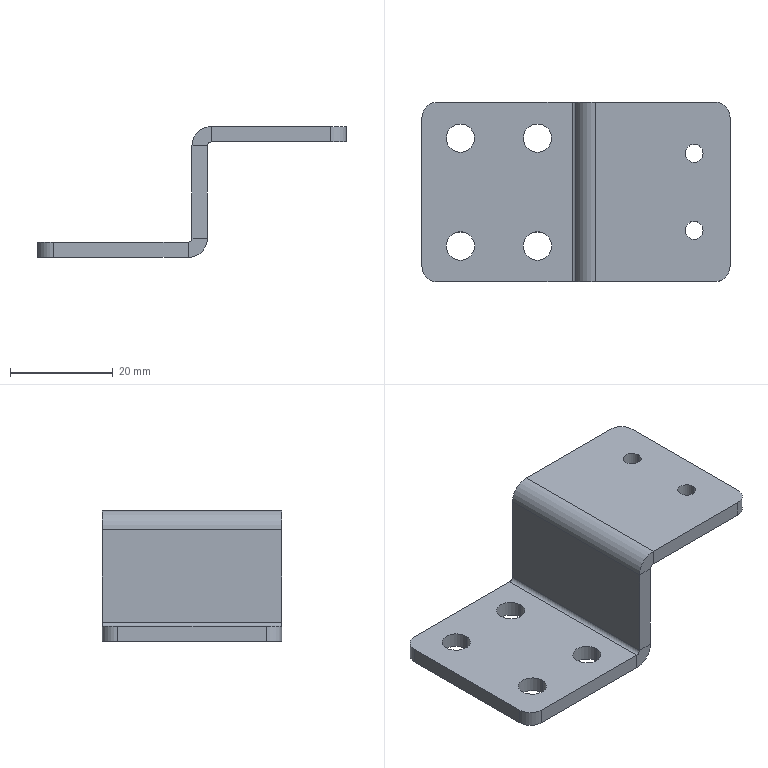Part | SolidWorks | features HoleWzd 2, Fillet 1, FlatPattern 1, SMBaseFlange 1, SheetMetal 1 | 1 solid | 38 faces | box 60 x 35 x 25.5 mm | volume 8094 mm3 | cylinder 20 | plane 18 | commonest cylinder face diameters 5.5 x8 3.5 x4 6 x4 1.5 x2 7.5 x2
STEP:
#1=CARTESIAN_POINT('',(-55.25,7.,-25.5));
#2=VERTEX_POINT('',#1);
#3=CARTESIAN_POINT('',(-49.75,7.,-25.5));
#4=VERTEX_POINT('',#3);
#5=CARTESIAN_POINT('',(-52.5,7.,-25.5));
#6=DIRECTION('',(0.,0.,1.));
#7=DIRECTION('',(1.,0.,0.));
#8=AXIS2_PLACEMENT_3D('',#5,#6,#7);
#9=CIRCLE('',#8,2.75);
#10=EDGE_CURVE('',#2,#4,#9,.T.);
#11=ORIENTED_EDGE('',*,*,#10,.F.);
#12=CARTESIAN_POINT('',(-55.25,7.,-22.5));
#13=VERTEX_POINT('',#12);
#14=CARTESIAN_POINT('',(-55.25,7.,-22.5));
#15=DIRECTION('',(0.,0.,1.));
#16=VECTOR('',#15,1000.);
#17=LINE('',#14,#16);
#18=EDGE_CURVE('',#2,#13,#17,.T.);
#19=ORIENTED_EDGE('',*,*,#18,.T.);
#20=CARTESIAN_POINT('',(-49.75,7.,-22.5));
#21=VERTEX_POINT('',#20);
#22=CARTESIAN_POINT('',(-52.5,7.,-22.5));
#23=DIRECTION('',(0.,0.,1.));
#24=DIRECTION('',(1.,0.,0.));
#25=AXIS2_PLACEMENT_3D('',#22,#23,#24);
#26=CIRCLE('',#25,2.75);
#27=EDGE_CURVE('',#13,#21,#26,.T.);
#28=ORIENTED_EDGE('',*,*,#27,.T.);
#29=CARTESIAN_POINT('',(-49.75,7.,-22.5));
#30=DIRECTION('',(0.,0.,1.));
#31=VECTOR('',#30,1000.);
#32=LINE('',#29,#31);
#33=EDGE_CURVE('',#4,#21,#32,.T.);
#34=ORIENTED_EDGE('',*,*,#33,.F.);
#35=EDGE_LOOP('',(#11,#19,#28,#34));
#36=FACE_OUTER_BOUND('',#35,.T.);
#37=CARTESIAN_POINT('',(-52.5,7.,-22.5));
#38=DIRECTION('',(0.,0.,1.));
#39=DIRECTION('',(1.,0.,0.));
#40=AXIS2_PLACEMENT_3D('',#37,#38,#39);
#41=CYLINDRICAL_SURFACE('',#40,2.75);
#42=ADVANCED_FACE('',(#36),#41,.F.);
#43=CARTESIAN_POINT('',(-40.25,7.,-25.5));
#44=VERTEX_POINT('',#43);
#45=CARTESIAN_POINT('',(-34.75,7.,-25.5));
#46=VERTEX_POINT('',#45);
#47=CARTESIAN_POINT('',(-37.5,7.,-25.5));
#48=DIRECTION('',(0.,0.,1.));
#49=DIRECTION('',(1.,0.,0.));
#50=AXIS2_PLACEMENT_3D('',#47,#48,#49);
#51=CIRCLE('',#50,2.75);
#52=EDGE_CURVE('',#44,#46,#51,.T.);
#53=ORIENTED_EDGE('',*,*,#52,.F.);
#54=CARTESIAN_POINT('',(-40.25,7.,-22.5));
#55=VERTEX_POINT('',#54);
#56=CARTESIAN_POINT('',(-40.25,7.,-22.5));
#57=DIRECTION('',(0.,0.,1.));
#58=VECTOR('',#57,1000.);
#59=LINE('',#56,#58);
#60=EDGE_CURVE('',#44,#55,#59,.T.);
#61=ORIENTED_EDGE('',*,*,#60,.T.);
#62=CARTESIAN_POINT('',(-34.75,7.,-22.5));
#63=VERTEX_POINT('',#62);
#64=CARTESIAN_POINT('',(-37.5,7.,-22.5));
#65=DIRECTION('',(0.,0.,1.));
#66=DIRECTION('',(1.,0.,0.));
#67=AXIS2_PLACEMENT_3D('',#64,#65,#66);
#68=CIRCLE('',#67,2.75);
#69=EDGE_CURVE('',#55,#63,#68,.T.);
#70=ORIENTED_EDGE('',*,*,#69,.T.);
#71=CARTESIAN_POINT('',(-34.75,7.,-22.5));
#72=DIRECTION('',(0.,0.,1.));
#73=VECTOR('',#72,1000.);
#74=LINE('',#71,#73);
#75=EDGE_CURVE('',#46,#63,#74,.T.);
#76=ORIENTED_EDGE('',*,*,#75,.F.);
#77=EDGE_LOOP('',(#53,#61,#70,#76));
#78=FACE_OUTER_BOUND('',#77,.T.);
#79=CARTESIAN_POINT('',(-37.5,7.,-22.5));
#80=DIRECTION('',(0.,0.,1.));
#81=DIRECTION('',(1.,0.,0.));
#82=AXIS2_PLACEMENT_3D('',#79,#80,#81);
#83=CYLINDRICAL_SURFACE('',#82,2.75);
#84=ADVANCED_FACE('',(#78),#83,.F.);
#85=CARTESIAN_POINT('',(-40.25,28.,-25.5));
#86=VERTEX_POINT('',#85);
#87=CARTESIAN_POINT('',(-34.75,28.,-25.5));
#88=VERTEX_POINT('',#87);
#89=CARTESIAN_POINT('',(-37.5,28.,-25.5));
#90=DIRECTION('',(0.,0.,1.));
#91=DIRECTION('',(1.,0.,0.));
#92=AXIS2_PLACEMENT_3D('',#89,#90,#91);
#93=CIRCLE('',#92,2.75);
#94=EDGE_CURVE('',#86,#88,#93,.T.);
#95=ORIENTED_EDGE('',*,*,#94,.F.);
#96=CARTESIAN_POINT('',(-40.25,28.,-22.5));
#97=VERTEX_POINT('',#96);
#98=CARTESIAN_POINT('',(-40.25,28.,-22.5));
#99=DIRECTION('',(0.,0.,1.));
#100=VECTOR('',#99,1000.);
#101=LINE('',#98,#100);
#102=EDGE_CURVE('',#86,#97,#101,.T.);
#103=ORIENTED_EDGE('',*,*,#102,.T.);
#104=CARTESIAN_POINT('',(-34.75,28.,-22.5));
#105=VERTEX_POINT('',#104);
#106=CARTESIAN_POINT('',(-37.5,28.,-22.5));
#107=DIRECTION('',(0.,0.,1.));
#108=DIRECTION('',(1.,0.,0.));
#109=AXIS2_PLACEMENT_3D('',#106,#107,#108);
#110=CIRCLE('',#109,2.75);
#111=EDGE_CURVE('',#97,#105,#110,.T.);
#112=ORIENTED_EDGE('',*,*,#111,.T.);
#113=CARTESIAN_POINT('',(-34.75,28.,-22.5));
#114=DIRECTION('',(0.,0.,1.));
#115=VECTOR('',#114,1000.);
#116=LINE('',#113,#115);
#117=EDGE_CURVE('',#88,#105,#116,.T.);
#118=ORIENTED_EDGE('',*,*,#117,.F.);
#119=EDGE_LOOP('',(#95,#103,#112,#118));
#120=FACE_OUTER_BOUND('',#119,.T.);
#121=CARTESIAN_POINT('',(-37.5,28.,-22.5));
#122=DIRECTION('',(0.,0.,1.));
#123=DIRECTION('',(1.,0.,0.));
#124=AXIS2_PLACEMENT_3D('',#121,#122,#123);
#125=CYLINDRICAL_SURFACE('',#124,2.75);
#126=ADVANCED_FACE('',(#120),#125,.F.);
#127=CARTESIAN_POINT('',(-55.25,28.,-25.5));
#128=VERTEX_POINT('',#127);
#129=CARTESIAN_POINT('',(-49.75,28.,-25.5));
#130=VERTEX_POINT('',#129);
#131=CARTESIAN_POINT('',(-52.5,28.,-25.5));
#132=DIRECTION('',(0.,0.,1.));
#133=DIRECTION('',(1.,0.,0.));
#134=AXIS2_PLACEMENT_3D('',#131,#132,#133);
#135=CIRCLE('',#134,2.75);
#136=EDGE_CURVE('',#128,#130,#135,.T.);
#137=ORIENTED_EDGE('',*,*,#136,.F.);
#138=CARTESIAN_POINT('',(-55.25,28.,-22.5));
#139=VERTEX_POINT('',#138);
#140=CARTESIAN_POINT('',(-55.25,28.,-22.5));
#141=DIRECTION('',(0.,0.,1.));
#142=VECTOR('',#141,1000.);
#143=LINE('',#140,#142);
#144=EDGE_CURVE('',#128,#139,#143,.T.);
#145=ORIENTED_EDGE('',*,*,#144,.T.);
#146=CARTESIAN_POINT('',(-49.75,28.,-22.5));
#147=VERTEX_POINT('',#146);
#148=CARTESIAN_POINT('',(-52.5,28.,-22.5));
#149=DIRECTION('',(0.,0.,1.));
#150=DIRECTION('',(1.,0.,0.));
#151=AXIS2_PLACEMENT_3D('',#148,#149,#150);
#152=CIRCLE('',#151,2.75);
#153=EDGE_CURVE('',#139,#147,#152,.T.);
#154=ORIENTED_EDGE('',*,*,#153,.T.);
#155=CARTESIAN_POINT('',(-49.75,28.,-22.5));
#156=DIRECTION('',(0.,0.,1.));
#157=VECTOR('',#156,1000.);
#158=LINE('',#155,#157);
#159=EDGE_CURVE('',#130,#147,#158,.T.);
#160=ORIENTED_EDGE('',*,*,#159,.F.);
#161=EDGE_LOOP('',(#137,#145,#154,#160));
#162=FACE_OUTER_BOUND('',#161,.T.);
#163=CARTESIAN_POINT('',(-52.5,28.,-22.5));
#164=DIRECTION('',(0.,0.,1.));
#165=DIRECTION('',(1.,0.,0.));
#166=AXIS2_PLACEMENT_3D('',#163,#164,#165);
#167=CYLINDRICAL_SURFACE('',#166,2.75);
#168=ADVANCED_FACE('',(#162),#167,.F.);
#169=CARTESIAN_POINT('',(-8.75,10.,0.));
#170=VERTEX_POINT('',#169);
#171=CARTESIAN_POINT('',(-5.25,10.,0.));
#172=VERTEX_POINT('',#171);
#173=CARTESIAN_POINT('',(-7.,10.,0.));
#174=DIRECTION('',(0.,0.,1.));
#175=DIRECTION('',(1.,0.,0.));
#176=AXIS2_PLACEMENT_3D('',#173,#174,#175);
#177=CIRCLE('',#176,1.75);
#178=EDGE_CURVE('',#170,#172,#177,.T.);
#179=ORIENTED_EDGE('',*,*,#178,.T.);
#180=CARTESIAN_POINT('',(-5.25,10.,-3.));
#181=VERTEX_POINT('',#180);
#182=CARTESIAN_POINT('',(-5.25,10.,-3.));
#183=DIRECTION('',(0.,0.,-1.));
#184=VECTOR('',#183,1000.);
#185=LINE('',#182,#184);
#186=EDGE_CURVE('',#172,#181,#185,.T.);
#187=ORIENTED_EDGE('',*,*,#186,.T.);
#188=CARTESIAN_POINT('',(-8.75,10.,-3.));
#189=VERTEX_POINT('',#188);
#190=CARTESIAN_POINT('',(-7.,10.,-3.));
#191=DIRECTION('',(0.,0.,-1.));
#192=DIRECTION('',(-1.,0.,0.));
#193=AXIS2_PLACEMENT_3D('',#190,#191,#192);
#194=CIRCLE('',#193,1.75);
#195=EDGE_CURVE('',#181,#189,#194,.T.);
#196=ORIENTED_EDGE('',*,*,#195,.T.);
#197=CARTESIAN_POINT('',(-8.75,10.,-3.));
#198=DIRECTION('',(0.,0.,-1.));
#199=VECTOR('',#198,1000.);
#200=LINE('',#197,#199);
#201=EDGE_CURVE('',#170,#189,#200,.T.);
#202=ORIENTED_EDGE('',*,*,#201,.F.);
#203=EDGE_LOOP('',(#179,#187,#196,#202));
#204=FACE_OUTER_BOUND('',#203,.T.);
#205=CARTESIAN_POINT('',(-7.,10.,-3.));
#206=DIRECTION('',(0.,0.,-1.));
#207=DIRECTION('',(-1.,0.,0.));
#208=AXIS2_PLACEMENT_3D('',#205,#206,#207);
#209=CYLINDRICAL_SURFACE('',#208,1.75);
#210=ADVANCED_FACE('',(#204),#209,.F.);
#211=CARTESIAN_POINT('',(-8.75,25.,0.));
#212=VERTEX_POINT('',#211);
#213=CARTESIAN_POINT('',(-5.25,25.,0.));
#214=VERTEX_POINT('',#213);
#215=CARTESIAN_POINT('',(-7.,25.,0.));
#216=DIRECTION('',(0.,0.,1.));
#217=DIRECTION('',(1.,0.,0.));
#218=AXIS2_PLACEMENT_3D('',#215,#216,#217);
#219=CIRCLE('',#218,1.75);
#220=EDGE_CURVE('',#212,#214,#219,.T.);
#221=ORIENTED_EDGE('',*,*,#220,.T.);
#222=CARTESIAN_POINT('',(-5.25,25.,-3.));
#223=VERTEX_POINT('',#222);
#224=CARTESIAN_POINT('',(-5.25,25.,-3.));
#225=DIRECTION('',(0.,0.,-1.));
#226=VECTOR('',#225,1000.);
#227=LINE('',#224,#226);
#228=EDGE_CURVE('',#214,#223,#227,.T.);
#229=ORIENTED_EDGE('',*,*,#228,.T.);
#230=CARTESIAN_POINT('',(-8.75,25.,-3.));
#231=VERTEX_POINT('',#230);
#232=CARTESIAN_POINT('',(-7.,25.,-3.));
#233=DIRECTION('',(0.,0.,-1.));
#234=DIRECTION('',(-1.,0.,0.));
#235=AXIS2_PLACEMENT_3D('',#232,#233,#234);
#236=CIRCLE('',#235,1.75);
#237=EDGE_CURVE('',#223,#231,#236,.T.);
#238=ORIENTED_EDGE('',*,*,#237,.T.);
#239=CARTESIAN_POINT('',(-8.75,25.,-3.));
#240=DIRECTION('',(0.,0.,-1.));
#241=VECTOR('',#240,1000.);
#242=LINE('',#239,#241);
#243=EDGE_CURVE('',#212,#231,#242,.T.);
#244=ORIENTED_EDGE('',*,*,#243,.F.);
#245=EDGE_LOOP('',(#221,#229,#238,#244));
#246=FACE_OUTER_BOUND('',#245,.T.);
#247=CARTESIAN_POINT('',(-7.,25.,-3.));
#248=DIRECTION('',(0.,0.,-1.));
#249=DIRECTION('',(-1.,0.,0.));
#250=AXIS2_PLACEMENT_3D('',#247,#248,#249);
#251=CYLINDRICAL_SURFACE('',#250,1.75);
#252=ADVANCED_FACE('',(#246),#251,.F.);
#253=CARTESIAN_POINT('',(-30.,35.,-3.75));
#254=VERTEX_POINT('',#253);
#255=CARTESIAN_POINT('',(-27.,35.,-3.75));
#256=VERTEX_POINT('',#255);
#257=CARTESIAN_POINT('',(-30.,35.,-3.75));
#258=DIRECTION('',(1.,0.,0.));
#259=VECTOR('',#258,1000.);
#260=LINE('',#257,#259);
#261=EDGE_CURVE('',#254,#256,#260,.T.);
#262=ORIENTED_EDGE('',*,*,#261,.F.);
#263=CARTESIAN_POINT('',(-26.25,35.,0.));
#264=VERTEX_POINT('',#263);
#265=CARTESIAN_POINT('',(-26.25,35.,-3.75));
#266=DIRECTION('',(0.,-1.,0.));
#267=DIRECTION('',(0.,0.,1.));
#268=AXIS2_PLACEMENT_3D('',#265,#266,#267);
#269=CIRCLE('',#268,3.75);
#270=EDGE_CURVE('',#264,#254,#269,.T.);
#271=ORIENTED_EDGE('',*,*,#270,.F.);
#272=CARTESIAN_POINT('',(-26.25,35.,-3.));
#273=VERTEX_POINT('',#272);
#274=CARTESIAN_POINT('',(-26.25,35.,-3.));
#275=DIRECTION('',(0.,0.,1.));
#276=VECTOR('',#275,1000.);
#277=LINE('',#274,#276);
#278=EDGE_CURVE('',#273,#264,#277,.T.);
#279=ORIENTED_EDGE('',*,*,#278,.F.);
#280=CARTESIAN_POINT('',(-26.25,35.,-3.75));
#281=DIRECTION('',(0.,-1.,0.));
#282=DIRECTION('',(1.,0.,0.));
#283=AXIS2_PLACEMENT_3D('',#280,#281,#282);
#284=CIRCLE('',#283,0.75);
#285=EDGE_CURVE('',#273,#256,#284,.T.);
#286=ORIENTED_EDGE('',*,*,#285,.T.);
#287=EDGE_LOOP('',(#262,#271,#279,#286));
#288=FACE_OUTER_BOUND('',#287,.T.);
#289=CARTESIAN_POINT('',(-30.,35.,-3.75));
#290=DIRECTION('',(0.,1.,0.));
#291=DIRECTION('',(0.,0.,1.));
#292=AXIS2_PLACEMENT_3D('',#289,#290,#291);
#293=PLANE('',#292);
#294=ADVANCED_FACE('',(#288),#293,.T.);
#295=CARTESIAN_POINT('',(-30.,35.,-21.75));
#296=VERTEX_POINT('',#295);
#297=CARTESIAN_POINT('',(-30.,35.,0.));
#298=DIRECTION('',(0.,0.,-1.));
#299=VECTOR('',#298,1000.);
#300=LINE('',#297,#299);
#301=EDGE_CURVE('',#254,#296,#300,.T.);
#302=ORIENTED_EDGE('',*,*,#301,.F.);
#303=ORIENTED_EDGE('',*,*,#261,.T.);
#304=CARTESIAN_POINT('',(-27.,35.,-21.75));
#305=VERTEX_POINT('',#304);
#306=CARTESIAN_POINT('',(-27.,35.,0.));
#307=DIRECTION('',(0.,0.,-1.));
#308=VECTOR('',#307,1000.);
#309=LINE('',#306,#308);
#310=EDGE_CURVE('',#256,#305,#309,.T.);
#311=ORIENTED_EDGE('',*,*,#310,.T.);
#312=CARTESIAN_POINT('',(-27.,35.,-21.75));
#313=DIRECTION('',(-1.,0.,0.));
#314=VECTOR('',#313,1000.);
#315=LINE('',#312,#314);
#316=EDGE_CURVE('',#305,#296,#315,.T.);
#317=ORIENTED_EDGE('',*,*,#316,.T.);
#318=EDGE_LOOP('',(#302,#303,#311,#317));
#319=FACE_OUTER_BOUND('',#318,.T.);
#320=CARTESIAN_POINT('',(-26.25,35.,-3.));
#321=DIRECTION('',(0.,1.,0.));
#322=DIRECTION('',(0.,0.,1.));
#323=AXIS2_PLACEMENT_3D('',#320,#321,#322);
#324=PLANE('',#323);
#325=ADVANCED_FACE('',(#319),#324,.T.);
#326=CARTESIAN_POINT('',(-26.25,0.,0.));
#327=VERTEX_POINT('',#326);
#328=CARTESIAN_POINT('',(-26.25,0.,-3.));
#329=VERTEX_POINT('',#328);
#330=CARTESIAN_POINT('',(-26.25,0.,0.));
#331=DIRECTION('',(0.,0.,-1.));
#332=VECTOR('',#331,1000.);
#333=LINE('',#330,#332);
#334=EDGE_CURVE('',#327,#329,#333,.T.);
#335=ORIENTED_EDGE('',*,*,#334,.F.);
#336=CARTESIAN_POINT('',(-30.,0.,-3.75));
#337=VERTEX_POINT('',#336);
#338=CARTESIAN_POINT('',(-26.25,0.,-3.75));
#339=DIRECTION('',(0.,-1.,0.));
#340=DIRECTION('',(0.,0.,1.));
#341=AXIS2_PLACEMENT_3D('',#338,#339,#340);
#342=CIRCLE('',#341,3.75);
#343=EDGE_CURVE('',#327,#337,#342,.T.);
#344=ORIENTED_EDGE('',*,*,#343,.T.);
#345=CARTESIAN_POINT('',(-27.,0.,-3.75));
#346=VERTEX_POINT('',#345);
#347=CARTESIAN_POINT('',(-27.,0.,-3.75));
#348=DIRECTION('',(-1.,0.,0.));
#349=VECTOR('',#348,1000.);
#350=LINE('',#347,#349);
#351=EDGE_CURVE('',#346,#337,#350,.T.);
#352=ORIENTED_EDGE('',*,*,#351,.F.);
#353=CARTESIAN_POINT('',(-26.25,0.,-3.75));
#354=DIRECTION('',(0.,-1.,0.));
#355=DIRECTION('',(1.,0.,0.));
#356=AXIS2_PLACEMENT_3D('',#353,#354,#355);
#357=CIRCLE('',#356,0.75);
#358=EDGE_CURVE('',#329,#346,#357,.T.);
#359=ORIENTED_EDGE('',*,*,#358,.F.);
#360=EDGE_LOOP('',(#335,#344,#352,#359));
#361=FACE_OUTER_BOUND('',#360,.T.);
#362=CARTESIAN_POINT('',(-26.25,0.,0.));
#363=DIRECTION('',(0.,-1.,0.));
#364=DIRECTION('',(0.,0.,-1.));
#365=AXIS2_PLACEMENT_3D('',#362,#363,#364);
#366=PLANE('',#365);
#367=ADVANCED_FACE('',(#361),#366,.T.);
#368=CARTESIAN_POINT('',(-3.,0.,-3.));
#369=VERTEX_POINT('',#368);
#370=CARTESIAN_POINT('',(0.,0.,-3.));
#371=DIRECTION('',(-1.,0.,0.));
#372=VECTOR('',#371,1000.);
#373=LINE('',#370,#372);
#374=EDGE_CURVE('',#369,#329,#373,.T.);
#375=ORIENTED_EDGE('',*,*,#374,.F.);
#376=CARTESIAN_POINT('',(-3.,0.,0.));
#377=VERTEX_POINT('',#376);
#378=CARTESIAN_POINT('',(-3.,0.,-3.75));
#379=DIRECTION('',(0.,0.,1.));
#380=VECTOR('',#379,1000.);
#381=LINE('',#378,#380);
#382=EDGE_CURVE('',#369,#377,#381,.T.);
#383=ORIENTED_EDGE('',*,*,#382,.T.);
#384=CARTESIAN_POINT('',(0.,0.,0.));
#385=DIRECTION('',(-1.,0.,0.));
#386=VECTOR('',#385,1000.);
#387=LINE('',#384,#386);
#388=EDGE_CURVE('',#377,#327,#387,.T.);
#389=ORIENTED_EDGE('',*,*,#388,.T.);
#390=ORIENTED_EDGE('',*,*,#334,.T.);
#391=EDGE_LOOP('',(#375,#383,#389,#390));
#392=FACE_OUTER_BOUND('',#391,.T.);
#393=CARTESIAN_POINT('',(-27.,0.,-3.75));
#394=DIRECTION('',(0.,-1.,0.));
#395=DIRECTION('',(0.,0.,-1.));
#396=AXIS2_PLACEMENT_3D('',#393,#394,#395);
#397=PLANE('',#396);
#398=ADVANCED_FACE('',(#392),#397,.T.);
#399=CARTESIAN_POINT('',(-30.75,35.,-22.5));
#400=VERTEX_POINT('',#399);
#401=CARTESIAN_POINT('',(-30.75,35.,-25.5));
#402=VERTEX_POINT('',#401);
#403=CARTESIAN_POINT('',(-30.75,35.,-22.5));
#404=DIRECTION('',(0.,0.,-1.));
#405=VECTOR('',#404,1000.);
#406=LINE('',#403,#405);
#407=EDGE_CURVE('',#400,#402,#406,.T.);
#408=ORIENTED_EDGE('',*,*,#407,.F.);
#409=CARTESIAN_POINT('',(-30.75,35.,-21.75));
#410=DIRECTION('',(0.,1.,0.));
#411=DIRECTION('',(0.,0.,-1.));
#412=AXIS2_PLACEMENT_3D('',#409,#410,#411);
#413=CIRCLE('',#412,0.75);
#414=EDGE_CURVE('',#296,#400,#413,.T.);
#415=ORIENTED_EDGE('',*,*,#414,.F.);
#416=ORIENTED_EDGE('',*,*,#316,.F.);
#417=CARTESIAN_POINT('',(-30.75,35.,-21.75));
#418=DIRECTION('',(0.,1.,0.));
#419=DIRECTION('',(1.,0.,0.));
#420=AXIS2_PLACEMENT_3D('',#417,#418,#419);
#421=CIRCLE('',#420,3.75);
#422=EDGE_CURVE('',#305,#402,#421,.T.);
#423=ORIENTED_EDGE('',*,*,#422,.T.);
#424=EDGE_LOOP('',(#408,#415,#416,#423));
#425=FACE_OUTER_BOUND('',#424,.T.);
#426=CARTESIAN_POINT('',(-30.75,35.,-22.5));
#427=DIRECTION('',(0.,1.,0.));
#428=DIRECTION('',(0.,0.,1.));
#429=AXIS2_PLACEMENT_3D('',#426,#427,#428);
#430=PLANE('',#429);
#431=ADVANCED_FACE('',(#425),#430,.T.);
#432=CARTESIAN_POINT('',(-57.,35.,-25.5));
#433=VERTEX_POINT('',#432);
#434=CARTESIAN_POINT('',(-30.,35.,-25.5));
#435=DIRECTION('',(-1.,0.,0.));
#436=VECTOR('',#435,1000.);
#437=LINE('',#434,#436);
#438=EDGE_CURVE('',#402,#433,#437,.T.);
#439=ORIENTED_EDGE('',*,*,#438,.T.);
#440=CARTESIAN_POINT('',(-57.,35.,-22.5));
#441=VERTEX_POINT('',#440);
#442=CARTESIAN_POINT('',(-57.,35.,-21.75));
#443=DIRECTION('',(0.,0.,1.));
#444=VECTOR('',#443,1000.);
#445=LINE('',#442,#444);
#446=EDGE_CURVE('',#433,#441,#445,.T.);
#447=ORIENTED_EDGE('',*,*,#446,.T.);
#448=CARTESIAN_POINT('',(-30.,35.,-22.5));
#449=DIRECTION('',(-1.,0.,0.));
#450=VECTOR('',#449,1000.);
#451=LINE('',#448,#450);
#452=EDGE_CURVE('',#400,#441,#451,.T.);
#453=ORIENTED_EDGE('',*,*,#452,.F.);
#454=ORIENTED_EDGE('',*,*,#407,.T.);
#455=EDGE_LOOP('',(#439,#447,#453,#454));
#456=FACE_OUTER_BOUND('',#455,.T.);
#457=CARTESIAN_POINT('',(-27.,35.,-21.75));
#458=DIRECTION('',(0.,1.,0.));
#459=DIRECTION('',(0.,0.,1.));
#460=AXIS2_PLACEMENT_3D('',#457,#458,#459);
#461=PLANE('',#460);
#462=ADVANCED_FACE('',(#456),#461,.T.);
#463=CARTESIAN_POINT('',(-30.,0.,-21.75));
#464=VERTEX_POINT('',#463);
#465=CARTESIAN_POINT('',(-27.,0.,-21.75));
#466=VERTEX_POINT('',#465);
#467=CARTESIAN_POINT('',(-30.,0.,-21.75));
#468=DIRECTION('',(1.,0.,0.));
#469=VECTOR('',#468,1000.);
#470=LINE('',#467,#469);
#471=EDGE_CURVE('',#464,#466,#470,.T.);
#472=ORIENTED_EDGE('',*,*,#471,.F.);
#473=CARTESIAN_POINT('',(-30.75,0.,-22.5));
#474=VERTEX_POINT('',#473);
#475=CARTESIAN_POINT('',(-30.75,0.,-21.75));
#476=DIRECTION('',(0.,1.,0.));
#477=DIRECTION('',(0.,0.,-1.));
#478=AXIS2_PLACEMENT_3D('',#475,#476,#477);
#479=CIRCLE('',#478,0.75);
#480=EDGE_CURVE('',#464,#474,#479,.T.);
#481=ORIENTED_EDGE('',*,*,#480,.T.);
#482=CARTESIAN_POINT('',(-30.75,0.,-25.5));
#483=VERTEX_POINT('',#482);
#484=CARTESIAN_POINT('',(-30.75,0.,-25.5));
#485=DIRECTION('',(0.,0.,1.));
#486=VECTOR('',#485,1000.);
#487=LINE('',#484,#486);
#488=EDGE_CURVE('',#483,#474,#487,.T.);
#489=ORIENTED_EDGE('',*,*,#488,.F.);
#490=CARTESIAN_POINT('',(-30.75,0.,-21.75));
#491=DIRECTION('',(0.,1.,0.));
#492=DIRECTION('',(1.,0.,0.));
#493=AXIS2_PLACEMENT_3D('',#490,#491,#492);
#494=CIRCLE('',#493,3.75);
#495=EDGE_CURVE('',#466,#483,#494,.T.);
#496=ORIENTED_EDGE('',*,*,#495,.F.);
#497=EDGE_LOOP('',(#472,#481,#489,#496));
#498=FACE_OUTER_BOUND('',#497,.T.);
#499=CARTESIAN_POINT('',(-30.,0.,-21.75));
#500=DIRECTION('',(0.,-1.,0.));
#501=DIRECTION('',(0.,0.,-1.));
#502=AXIS2_PLACEMENT_3D('',#499,#500,#501);
#503=PLANE('',#502);
#504=ADVANCED_FACE('',(#498),#503,.T.);
#505=CARTESIAN_POINT('',(-30.,0.,0.));
#506=DIRECTION('',(0.,0.,-1.));
#507=VECTOR('',#506,1000.);
#508=LINE('',#505,#507);
#509=EDGE_CURVE('',#337,#464,#508,.T.);
#510=ORIENTED_EDGE('',*,*,#509,.T.);
#511=ORIENTED_EDGE('',*,*,#471,.T.);
#512=CARTESIAN_POINT('',(-27.,0.,0.));
#513=DIRECTION('',(0.,0.,-1.));
#514=VECTOR('',#513,1000.);
#515=LINE('',#512,#514);
#516=EDGE_CURVE('',#346,#466,#515,.T.);
#517=ORIENTED_EDGE('',*,*,#516,.F.);
#518=ORIENTED_EDGE('',*,*,#351,.T.);
#519=EDGE_LOOP('',(#510,#511,#517,#518));
#520=FACE_OUTER_BOUND('',#519,.T.);
#521=CARTESIAN_POINT('',(-30.75,0.,-25.5));
#522=DIRECTION('',(0.,-1.,0.));
#523=DIRECTION('',(0.,0.,-1.));
#524=AXIS2_PLACEMENT_3D('',#521,#522,#523);
#525=PLANE('',#524);
#526=ADVANCED_FACE('',(#520),#525,.T.);
#527=CARTESIAN_POINT('',(-52.5,7.,-25.5));
#528=DIRECTION('',(0.,0.,1.));
#529=DIRECTION('',(1.,0.,0.));
#530=AXIS2_PLACEMENT_3D('',#527,#528,#529);
#531=CIRCLE('',#530,2.75);
#532=EDGE_CURVE('',#4,#2,#531,.T.);
#533=ORIENTED_EDGE('',*,*,#532,.T.);
#534=ORIENTED_EDGE('',*,*,#10,.T.);
#535=EDGE_LOOP('',(#533,#534));
#536=FACE_BOUND('',#535,.T.);
#537=CARTESIAN_POINT('',(-37.5,7.,-25.5));
#538=DIRECTION('',(0.,0.,1.));
#539=DIRECTION('',(1.,0.,0.));
#540=AXIS2_PLACEMENT_3D('',#537,#538,#539);
#541=CIRCLE('',#540,2.75);
#542=EDGE_CURVE('',#46,#44,#541,.T.);
#543=ORIENTED_EDGE('',*,*,#542,.T.);
#544=ORIENTED_EDGE('',*,*,#52,.T.);
#545=EDGE_LOOP('',(#543,#544));
#546=FACE_BOUND('',#545,.T.);
#547=CARTESIAN_POINT('',(-37.5,28.,-25.5));
#548=DIRECTION('',(0.,0.,1.));
#549=DIRECTION('',(1.,0.,0.));
#550=AXIS2_PLACEMENT_3D('',#547,#548,#549);
#551=CIRCLE('',#550,2.75);
#552=EDGE_CURVE('',#88,#86,#551,.T.);
#553=ORIENTED_EDGE('',*,*,#552,.T.);
#554=ORIENTED_EDGE('',*,*,#94,.T.);
#555=EDGE_LOOP('',(#553,#554));
#556=FACE_BOUND('',#555,.T.);
#557=CARTESIAN_POINT('',(-52.5,28.,-25.5));
#558=DIRECTION('',(0.,0.,1.));
#559=DIRECTION('',(1.,0.,0.));
#560=AXIS2_PLACEMENT_3D('',#557,#558,#559);
#561=CIRCLE('',#560,2.75);
#562=EDGE_CURVE('',#130,#128,#561,.T.);
#563=ORIENTED_EDGE('',*,*,#562,.T.);
#564=ORIENTED_EDGE('',*,*,#136,.T.);
#565=EDGE_LOOP('',(#563,#564));
#566=FACE_BOUND('',#565,.T.);
#567=CARTESIAN_POINT('',(-57.,0.,-25.5));
#568=VERTEX_POINT('',#567);
#569=CARTESIAN_POINT('',(-30.,0.,-25.5));
#570=DIRECTION('',(-1.,0.,0.));
#571=VECTOR('',#570,1000.);
#572=LINE('',#569,#571);
#573=EDGE_CURVE('',#483,#568,#572,.T.);
#574=ORIENTED_EDGE('',*,*,#573,.T.);
#575=CARTESIAN_POINT('',(-60.,3.,-25.5));
#576=VERTEX_POINT('',#575);
#577=CARTESIAN_POINT('',(-57.,3.,-25.5));
#578=DIRECTION('',(0.,0.,-1.));
#579=DIRECTION('',(1.,0.,0.));
#580=AXIS2_PLACEMENT_3D('',#577,#578,#579);
#581=CIRCLE('',#580,3.);
#582=EDGE_CURVE('',#568,#576,#581,.T.);
#583=ORIENTED_EDGE('',*,*,#582,.T.);
#584=CARTESIAN_POINT('',(-60.,32.,-25.5));
#585=VERTEX_POINT('',#584);
#586=CARTESIAN_POINT('',(-60.,35.,-25.5));
#587=DIRECTION('',(0.,-1.,0.));
#588=VECTOR('',#587,1000.);
#589=LINE('',#586,#588);
#590=EDGE_CURVE('',#585,#576,#589,.T.);
#591=ORIENTED_EDGE('',*,*,#590,.F.);
#592=CARTESIAN_POINT('',(-57.,32.,-25.5));
#593=DIRECTION('',(0.,0.,-1.));
#594=DIRECTION('',(1.,0.,0.));
#595=AXIS2_PLACEMENT_3D('',#592,#593,#594);
#596=CIRCLE('',#595,3.);
#597=EDGE_CURVE('',#585,#433,#596,.T.);
#598=ORIENTED_EDGE('',*,*,#597,.T.);
#599=ORIENTED_EDGE('',*,*,#438,.F.);
#600=CARTESIAN_POINT('',(-30.75,35.,-25.5));
#601=DIRECTION('',(0.,-1.,0.));
#602=VECTOR('',#601,1000.);
#603=LINE('',#600,#602);
#604=EDGE_CURVE('',#402,#483,#603,.T.);
#605=ORIENTED_EDGE('',*,*,#604,.T.);
#606=EDGE_LOOP('',(#574,#583,#591,#598,#599,#605));
#607=FACE_OUTER_BOUND('',#606,.T.);
#608=CARTESIAN_POINT('',(-30.,35.,-25.5));
#609=DIRECTION('',(0.,0.,1.));
#610=DIRECTION('',(1.,0.,0.));
#611=AXIS2_PLACEMENT_3D('',#608,#609,#610);
#612=PLANE('',#611);
#613=ADVANCED_FACE('',(#536,#546,#556,#566,#607),#612,.F.);
#614=ORIENTED_EDGE('',*,*,#590,.T.);
#615=CARTESIAN_POINT('',(-60.,3.,-22.5));
#616=VERTEX_POINT('',#615);
#617=CARTESIAN_POINT('',(-60.,3.,-22.5));
#618=DIRECTION('',(0.,0.,1.));
#619=VECTOR('',#618,1000.);
#620=LINE('',#617,#619);
#621=EDGE_CURVE('',#576,#616,#620,.T.);
#622=ORIENTED_EDGE('',*,*,#621,.T.);
#623=CARTESIAN_POINT('',(-60.,32.,-22.5));
#624=VERTEX_POINT('',#623);
#625=CARTESIAN_POINT('',(-60.,35.,-22.5));
#626=DIRECTION('',(0.,-1.,0.));
#627=VECTOR('',#626,1000.);
#628=LINE('',#625,#627);
#629=EDGE_CURVE('',#624,#616,#628,.T.);
#630=ORIENTED_EDGE('',*,*,#629,.F.);
#631=CARTESIAN_POINT('',(-60.,32.,-22.5));
#632=DIRECTION('',(0.,0.,-1.));
#633=VECTOR('',#632,1000.);
#634=LINE('',#631,#633);
#635=EDGE_CURVE('',#624,#585,#634,.T.);
#636=ORIENTED_EDGE('',*,*,#635,.T.);
#637=EDGE_LOOP('',(#614,#622,#630,#636));
#638=FACE_OUTER_BOUND('',#637,.T.);
#639=CARTESIAN_POINT('',(-60.,35.,-22.5));
#640=DIRECTION('',(-1.,0.,0.));
#641=DIRECTION('',(0.,0.,1.));
#642=AXIS2_PLACEMENT_3D('',#639,#640,#641);
#643=PLANE('',#642);
#644=ADVANCED_FACE('',(#638),#643,.T.);
#645=CARTESIAN_POINT('',(-52.5,7.,-22.5));
#646=DIRECTION('',(0.,0.,1.));
#647=DIRECTION('',(1.,0.,0.));
#648=AXIS2_PLACEMENT_3D('',#645,#646,#647);
#649=CIRCLE('',#648,2.75);
#650=EDGE_CURVE('',#21,#13,#649,.T.);
#651=ORIENTED_EDGE('',*,*,#650,.F.);
#652=ORIENTED_EDGE('',*,*,#27,.F.);
#653=EDGE_LOOP('',(#651,#652));
#654=FACE_BOUND('',#653,.T.);
#655=CARTESIAN_POINT('',(-37.5,7.,-22.5));
#656=DIRECTION('',(0.,0.,1.));
#657=DIRECTION('',(1.,0.,0.));
#658=AXIS2_PLACEMENT_3D('',#655,#656,#657);
#659=CIRCLE('',#658,2.75);
#660=EDGE_CURVE('',#63,#55,#659,.T.);
#661=ORIENTED_EDGE('',*,*,#660,.F.);
#662=ORIENTED_EDGE('',*,*,#69,.F.);
#663=EDGE_LOOP('',(#661,#662));
#664=FACE_BOUND('',#663,.T.);
#665=CARTESIAN_POINT('',(-37.5,28.,-22.5));
#666=DIRECTION('',(0.,0.,1.));
#667=DIRECTION('',(1.,0.,0.));
#668=AXIS2_PLACEMENT_3D('',#665,#666,#667);
#669=CIRCLE('',#668,2.75);
#670=EDGE_CURVE('',#105,#97,#669,.T.);
#671=ORIENTED_EDGE('',*,*,#670,.F.);
#672=ORIENTED_EDGE('',*,*,#111,.F.);
#673=EDGE_LOOP('',(#671,#672));
#674=FACE_BOUND('',#673,.T.);
#675=CARTESIAN_POINT('',(-52.5,28.,-22.5));
#676=DIRECTION('',(0.,0.,1.));
#677=DIRECTION('',(1.,0.,0.));
#678=AXIS2_PLACEMENT_3D('',#675,#676,#677);
#679=CIRCLE('',#678,2.75);
#680=EDGE_CURVE('',#147,#139,#679,.T.);
#681=ORIENTED_EDGE('',*,*,#680,.F.);
#682=ORIENTED_EDGE('',*,*,#153,.F.);
#683=EDGE_LOOP('',(#681,#682));
#684=FACE_BOUND('',#683,.T.);
#685=ORIENTED_EDGE('',*,*,#629,.T.);
#686=CARTESIAN_POINT('',(-57.,0.,-22.5));
#687=VERTEX_POINT('',#686);
#688=CARTESIAN_POINT('',(-57.,3.,-22.5));
#689=DIRECTION('',(0.,0.,1.));
#690=DIRECTION('',(1.,0.,0.));
#691=AXIS2_PLACEMENT_3D('',#688,#689,#690);
#692=CIRCLE('',#691,3.);
#693=EDGE_CURVE('',#616,#687,#692,.T.);
#694=ORIENTED_EDGE('',*,*,#693,.T.);
#695=CARTESIAN_POINT('',(-30.,0.,-22.5));
#696=DIRECTION('',(-1.,0.,0.));
#697=VECTOR('',#696,1000.);
#698=LINE('',#695,#697);
#699=EDGE_CURVE('',#474,#687,#698,.T.);
#700=ORIENTED_EDGE('',*,*,#699,.F.);
#701=CARTESIAN_POINT('',(-30.75,35.,-22.5));
#702=DIRECTION('',(0.,-1.,0.));
#703=VECTOR('',#702,1000.);
#704=LINE('',#701,#703);
#705=EDGE_CURVE('',#400,#474,#704,.T.);
#706=ORIENTED_EDGE('',*,*,#705,.F.);
#707=ORIENTED_EDGE('',*,*,#452,.T.);
#708=CARTESIAN_POINT('',(-57.,32.,-22.5));
#709=DIRECTION('',(0.,0.,1.));
#710=DIRECTION('',(1.,0.,0.));
#711=AXIS2_PLACEMENT_3D('',#708,#709,#710);
#712=CIRCLE('',#711,3.);
#713=EDGE_CURVE('',#441,#624,#712,.T.);
#714=ORIENTED_EDGE('',*,*,#713,.T.);
#715=EDGE_LOOP('',(#685,#694,#700,#706,#707,#714));
#716=FACE_OUTER_BOUND('',#715,.T.);
#717=CARTESIAN_POINT('',(-30.,35.,-22.5));
#718=DIRECTION('',(0.,0.,1.));
#719=DIRECTION('',(1.,0.,0.));
#720=AXIS2_PLACEMENT_3D('',#717,#718,#719);
#721=PLANE('',#720);
#722=ADVANCED_FACE('',(#654,#664,#674,#684,#716),#721,.T.);
#723=ORIENTED_EDGE('',*,*,#480,.F.);
#724=CARTESIAN_POINT('',(-30.,35.,-21.75));
#725=DIRECTION('',(0.,-1.,0.));
#726=VECTOR('',#725,1000.);
#727=LINE('',#724,#726);
#728=EDGE_CURVE('',#296,#464,#727,.T.);
#729=ORIENTED_EDGE('',*,*,#728,.F.);
#730=ORIENTED_EDGE('',*,*,#414,.T.);
#731=ORIENTED_EDGE('',*,*,#705,.T.);
#732=EDGE_LOOP('',(#723,#729,#730,#731));
#733=FACE_OUTER_BOUND('',#732,.T.);
#734=CARTESIAN_POINT('',(-30.75,35.,-21.75));
#735=DIRECTION('',(0.,-1.,0.));
#736=DIRECTION('',(0.,0.,-1.));
#737=AXIS2_PLACEMENT_3D('',#734,#735,#736);
#738=CYLINDRICAL_SURFACE('',#737,0.75);
#739=ADVANCED_FACE('',(#733),#738,.F.);
#740=ORIENTED_EDGE('',*,*,#509,.F.);
#741=CARTESIAN_POINT('',(-30.,35.,-3.75));
#742=DIRECTION('',(0.,-1.,0.));
#743=VECTOR('',#742,1000.);
#744=LINE('',#741,#743);
#745=EDGE_CURVE('',#254,#337,#744,.T.);
#746=ORIENTED_EDGE('',*,*,#745,.F.);
#747=ORIENTED_EDGE('',*,*,#301,.T.);
#748=ORIENTED_EDGE('',*,*,#728,.T.);
#749=EDGE_LOOP('',(#740,#746,#747,#748));
#750=FACE_OUTER_BOUND('',#749,.T.);
#751=CARTESIAN_POINT('',(-30.,35.,0.));
#752=DIRECTION('',(-1.,0.,0.));
#753=DIRECTION('',(0.,0.,1.));
#754=AXIS2_PLACEMENT_3D('',#751,#752,#753);
#755=PLANE('',#754);
#756=ADVANCED_FACE('',(#750),#755,.T.);
#757=ORIENTED_EDGE('',*,*,#343,.F.);
#758=CARTESIAN_POINT('',(-26.25,35.,0.));
#759=DIRECTION('',(0.,-1.,0.));
#760=VECTOR('',#759,1000.);
#761=LINE('',#758,#760);
#762=EDGE_CURVE('',#264,#327,#761,.T.);
#763=ORIENTED_EDGE('',*,*,#762,.F.);
#764=ORIENTED_EDGE('',*,*,#270,.T.);
#765=ORIENTED_EDGE('',*,*,#745,.T.);
#766=EDGE_LOOP('',(#757,#763,#764,#765));
#767=FACE_OUTER_BOUND('',#766,.T.);
#768=CARTESIAN_POINT('',(-26.25,35.,-3.75));
#769=DIRECTION('',(0.,-1.,0.));
#770=DIRECTION('',(0.,0.,-1.));
#771=AXIS2_PLACEMENT_3D('',#768,#769,#770);
#772=CYLINDRICAL_SURFACE('',#771,3.75);
#773=ADVANCED_FACE('',(#767),#772,.T.);
#774=ORIENTED_EDGE('',*,*,#178,.F.);
#775=CARTESIAN_POINT('',(-7.,10.,0.));
#776=DIRECTION('',(0.,0.,1.));
#777=DIRECTION('',(1.,0.,0.));
#778=AXIS2_PLACEMENT_3D('',#775,#776,#777);
#779=CIRCLE('',#778,1.75);
#780=EDGE_CURVE('',#172,#170,#779,.T.);
#781=ORIENTED_EDGE('',*,*,#780,.F.);
#782=EDGE_LOOP('',(#774,#781));
#783=FACE_BOUND('',#782,.T.);
#784=ORIENTED_EDGE('',*,*,#220,.F.);
#785=CARTESIAN_POINT('',(-7.,25.,0.));
#786=DIRECTION('',(0.,0.,1.));
#787=DIRECTION('',(1.,0.,0.));
#788=AXIS2_PLACEMENT_3D('',#785,#786,#787);
#789=CIRCLE('',#788,1.75);
#790=EDGE_CURVE('',#214,#212,#789,.T.);
#791=ORIENTED_EDGE('',*,*,#790,.F.);
#792=EDGE_LOOP('',(#784,#791));
#793=FACE_BOUND('',#792,.T.);
#794=ORIENTED_EDGE('',*,*,#388,.F.);
#795=CARTESIAN_POINT('',(0.,3.,0.));
#796=VERTEX_POINT('',#795);
#797=CARTESIAN_POINT('',(-3.,3.,0.));
#798=DIRECTION('',(0.,0.,1.));
#799=DIRECTION('',(1.,0.,0.));
#800=AXIS2_PLACEMENT_3D('',#797,#798,#799);
#801=CIRCLE('',#800,3.);
#802=EDGE_CURVE('',#377,#796,#801,.T.);
#803=ORIENTED_EDGE('',*,*,#802,.T.);
#804=CARTESIAN_POINT('',(0.,32.,0.));
#805=VERTEX_POINT('',#804);
#806=CARTESIAN_POINT('',(0.,35.,0.));
#807=DIRECTION('',(0.,-1.,0.));
#808=VECTOR('',#807,1000.);
#809=LINE('',#806,#808);
#810=EDGE_CURVE('',#805,#796,#809,.T.);
#811=ORIENTED_EDGE('',*,*,#810,.F.);
#812=CARTESIAN_POINT('',(-3.,35.,0.));
#813=VERTEX_POINT('',#812);
#814=CARTESIAN_POINT('',(-3.,32.,0.));
#815=DIRECTION('',(0.,0.,1.));
#816=DIRECTION('',(1.,0.,0.));
#817=AXIS2_PLACEMENT_3D('',#814,#815,#816);
#818=CIRCLE('',#817,3.);
#819=EDGE_CURVE('',#805,#813,#818,.T.);
#820=ORIENTED_EDGE('',*,*,#819,.T.);
#821=CARTESIAN_POINT('',(0.,35.,0.));
#822=DIRECTION('',(-1.,0.,0.));
#823=VECTOR('',#822,1000.);
#824=LINE('',#821,#823);
#825=EDGE_CURVE('',#813,#264,#824,.T.);
#826=ORIENTED_EDGE('',*,*,#825,.T.);
#827=ORIENTED_EDGE('',*,*,#762,.T.);
#828=EDGE_LOOP('',(#794,#803,#811,#820,#826,#827));
#829=FACE_OUTER_BOUND('',#828,.T.);
#830=CARTESIAN_POINT('',(0.,35.,0.));
#831=DIRECTION('',(0.,0.,1.));
#832=DIRECTION('',(1.,0.,0.));
#833=AXIS2_PLACEMENT_3D('',#830,#831,#832);
#834=PLANE('',#833);
#835=ADVANCED_FACE('',(#783,#793,#829),#834,.T.);
#836=ORIENTED_EDGE('',*,*,#810,.T.);
#837=CARTESIAN_POINT('',(0.,3.,-3.));
#838=VERTEX_POINT('',#837);
#839=CARTESIAN_POINT('',(0.,3.,-3.));
#840=DIRECTION('',(0.,0.,-1.));
#841=VECTOR('',#840,1000.);
#842=LINE('',#839,#841);
#843=EDGE_CURVE('',#796,#838,#842,.T.);
#844=ORIENTED_EDGE('',*,*,#843,.T.);
#845=CARTESIAN_POINT('',(0.,32.,-3.));
#846=VERTEX_POINT('',#845);
#847=CARTESIAN_POINT('',(0.,35.,-3.));
#848=DIRECTION('',(0.,-1.,0.));
#849=VECTOR('',#848,1000.);
#850=LINE('',#847,#849);
#851=EDGE_CURVE('',#846,#838,#850,.T.);
#852=ORIENTED_EDGE('',*,*,#851,.F.);
#853=CARTESIAN_POINT('',(0.,32.,0.));
#854=DIRECTION('',(0.,0.,1.));
#855=VECTOR('',#854,1000.);
#856=LINE('',#853,#855);
#857=EDGE_CURVE('',#846,#805,#856,.T.);
#858=ORIENTED_EDGE('',*,*,#857,.T.);
#859=EDGE_LOOP('',(#836,#844,#852,#858));
#860=FACE_OUTER_BOUND('',#859,.T.);
#861=CARTESIAN_POINT('',(0.,35.,-3.));
#862=DIRECTION('',(1.,0.,0.));
#863=DIRECTION('',(0.,0.,-1.));
#864=AXIS2_PLACEMENT_3D('',#861,#862,#863);
#865=PLANE('',#864);
#866=ADVANCED_FACE('',(#860),#865,.T.);
#867=CARTESIAN_POINT('',(-7.,10.,-3.));
#868=DIRECTION('',(0.,0.,-1.));
#869=DIRECTION('',(-1.,0.,0.));
#870=AXIS2_PLACEMENT_3D('',#867,#868,#869);
#871=CIRCLE('',#870,1.75);
#872=EDGE_CURVE('',#189,#181,#871,.T.);
#873=ORIENTED_EDGE('',*,*,#872,.F.);
#874=ORIENTED_EDGE('',*,*,#195,.F.);
#875=EDGE_LOOP('',(#873,#874));
#876=FACE_BOUND('',#875,.T.);
#877=CARTESIAN_POINT('',(-7.,25.,-3.));
#878=DIRECTION('',(0.,0.,-1.));
#879=DIRECTION('',(-1.,0.,0.));
#880=AXIS2_PLACEMENT_3D('',#877,#878,#879);
#881=CIRCLE('',#880,1.75);
#882=EDGE_CURVE('',#231,#223,#881,.T.);
#883=ORIENTED_EDGE('',*,*,#882,.F.);
#884=ORIENTED_EDGE('',*,*,#237,.F.);
#885=EDGE_LOOP('',(#883,#884));
#886=FACE_BOUND('',#885,.T.);
#887=ORIENTED_EDGE('',*,*,#851,.T.);
#888=CARTESIAN_POINT('',(-3.,3.,-3.));
#889=DIRECTION('',(0.,0.,-1.));
#890=DIRECTION('',(1.,0.,0.));
#891=AXIS2_PLACEMENT_3D('',#888,#889,#890);
#892=CIRCLE('',#891,3.);
#893=EDGE_CURVE('',#838,#369,#892,.T.);
#894=ORIENTED_EDGE('',*,*,#893,.T.);
#895=ORIENTED_EDGE('',*,*,#374,.T.);
#896=CARTESIAN_POINT('',(-26.25,35.,-3.));
#897=DIRECTION('',(0.,-1.,0.));
#898=VECTOR('',#897,1000.);
#899=LINE('',#896,#898);
#900=EDGE_CURVE('',#273,#329,#899,.T.);
#901=ORIENTED_EDGE('',*,*,#900,.F.);
#902=CARTESIAN_POINT('',(-3.,35.,-3.));
#903=VERTEX_POINT('',#902);
#904=CARTESIAN_POINT('',(0.,35.,-3.));
#905=DIRECTION('',(-1.,0.,0.));
#906=VECTOR('',#905,1000.);
#907=LINE('',#904,#906);
#908=EDGE_CURVE('',#903,#273,#907,.T.);
#909=ORIENTED_EDGE('',*,*,#908,.F.);
#910=CARTESIAN_POINT('',(-3.,32.,-3.));
#911=DIRECTION('',(0.,0.,-1.));
#912=DIRECTION('',(1.,0.,0.));
#913=AXIS2_PLACEMENT_3D('',#910,#911,#912);
#914=CIRCLE('',#913,3.);
#915=EDGE_CURVE('',#903,#846,#914,.T.);
#916=ORIENTED_EDGE('',*,*,#915,.T.);
#917=EDGE_LOOP('',(#887,#894,#895,#901,#909,#916));
#918=FACE_OUTER_BOUND('',#917,.T.);
#919=CARTESIAN_POINT('',(0.,35.,-3.));
#920=DIRECTION('',(0.,0.,1.));
#921=DIRECTION('',(1.,0.,0.));
#922=AXIS2_PLACEMENT_3D('',#919,#920,#921);
#923=PLANE('',#922);
#924=ADVANCED_FACE('',(#876,#886,#918),#923,.F.);
#925=ORIENTED_EDGE('',*,*,#358,.T.);
#926=CARTESIAN_POINT('',(-27.,35.,-3.75));
#927=DIRECTION('',(0.,-1.,0.));
#928=VECTOR('',#927,1000.);
#929=LINE('',#926,#928);
#930=EDGE_CURVE('',#256,#346,#929,.T.);
#931=ORIENTED_EDGE('',*,*,#930,.F.);
#932=ORIENTED_EDGE('',*,*,#285,.F.);
#933=ORIENTED_EDGE('',*,*,#900,.T.);
#934=EDGE_LOOP('',(#925,#931,#932,#933));
#935=FACE_OUTER_BOUND('',#934,.T.);
#936=CARTESIAN_POINT('',(-26.25,35.,-3.75));
#937=DIRECTION('',(0.,-1.,0.));
#938=DIRECTION('',(0.,0.,-1.));
#939=AXIS2_PLACEMENT_3D('',#936,#937,#938);
#940=CYLINDRICAL_SURFACE('',#939,0.75);
#941=ADVANCED_FACE('',(#935),#940,.F.);
#942=ORIENTED_EDGE('',*,*,#516,.T.);
#943=CARTESIAN_POINT('',(-27.,35.,-21.75));
#944=DIRECTION('',(0.,-1.,0.));
#945=VECTOR('',#944,1000.);
#946=LINE('',#943,#945);
#947=EDGE_CURVE('',#305,#466,#946,.T.);
#948=ORIENTED_EDGE('',*,*,#947,.F.);
#949=ORIENTED_EDGE('',*,*,#310,.F.);
#950=ORIENTED_EDGE('',*,*,#930,.T.);
#951=EDGE_LOOP('',(#942,#948,#949,#950));
#952=FACE_OUTER_BOUND('',#951,.T.);
#953=CARTESIAN_POINT('',(-27.,35.,0.));
#954=DIRECTION('',(-1.,0.,0.));
#955=DIRECTION('',(0.,0.,1.));
#956=AXIS2_PLACEMENT_3D('',#953,#954,#955);
#957=PLANE('',#956);
#958=ADVANCED_FACE('',(#952),#957,.F.);
#959=ORIENTED_EDGE('',*,*,#495,.T.);
#960=ORIENTED_EDGE('',*,*,#604,.F.);
#961=ORIENTED_EDGE('',*,*,#422,.F.);
#962=ORIENTED_EDGE('',*,*,#947,.T.);
#963=EDGE_LOOP('',(#959,#960,#961,#962));
#964=FACE_OUTER_BOUND('',#963,.T.);
#965=CARTESIAN_POINT('',(-30.75,35.,-21.75));
#966=DIRECTION('',(0.,-1.,0.));
#967=DIRECTION('',(0.,0.,-1.));
#968=AXIS2_PLACEMENT_3D('',#965,#966,#967);
#969=CYLINDRICAL_SURFACE('',#968,3.75);
#970=ADVANCED_FACE('',(#964),#969,.T.);
#971=ORIENTED_EDGE('',*,*,#825,.F.);
#972=CARTESIAN_POINT('',(-3.,35.,-3.));
#973=DIRECTION('',(0.,0.,-1.));
#974=VECTOR('',#973,1000.);
#975=LINE('',#972,#974);
#976=EDGE_CURVE('',#813,#903,#975,.T.);
#977=ORIENTED_EDGE('',*,*,#976,.T.);
#978=ORIENTED_EDGE('',*,*,#908,.T.);
#979=ORIENTED_EDGE('',*,*,#278,.T.);
#980=EDGE_LOOP('',(#971,#977,#978,#979));
#981=FACE_OUTER_BOUND('',#980,.T.);
#982=CARTESIAN_POINT('',(-30.75,35.,-21.75));
#983=DIRECTION('',(0.,-1.,0.));
#984=DIRECTION('',(-1.,0.,0.));
#985=AXIS2_PLACEMENT_3D('',#982,#983,#984);
#986=PLANE('',#985);
#987=ADVANCED_FACE('',(#981),#986,.F.);
#988=ORIENTED_EDGE('',*,*,#699,.T.);
#989=CARTESIAN_POINT('',(-57.,0.,-21.75));
#990=DIRECTION('',(0.,0.,-1.));
#991=VECTOR('',#990,1000.);
#992=LINE('',#989,#991);
#993=EDGE_CURVE('',#687,#568,#992,.T.);
#994=ORIENTED_EDGE('',*,*,#993,.T.);
#995=ORIENTED_EDGE('',*,*,#573,.F.);
#996=ORIENTED_EDGE('',*,*,#488,.T.);
#997=EDGE_LOOP('',(#988,#994,#995,#996));
#998=FACE_OUTER_BOUND('',#997,.T.);
#999=CARTESIAN_POINT('',(-30.75,0.,-21.75));
#1000=DIRECTION('',(0.,-1.,0.));
#1001=DIRECTION('',(-1.,0.,0.));
#1002=AXIS2_PLACEMENT_3D('',#999,#1000,#1001);
#1003=PLANE('',#1002);
#1004=ADVANCED_FACE('',(#998),#1003,.T.);
#1005=ORIENTED_EDGE('',*,*,#893,.F.);
#1006=ORIENTED_EDGE('',*,*,#843,.F.);
#1007=ORIENTED_EDGE('',*,*,#802,.F.);
#1008=ORIENTED_EDGE('',*,*,#382,.F.);
#1009=EDGE_LOOP('',(#1005,#1006,#1007,#1008));
#1010=FACE_OUTER_BOUND('',#1009,.T.);
#1011=CARTESIAN_POINT('',(-3.,3.,-3.75));
#1012=DIRECTION('',(0.,0.,1.));
#1013=DIRECTION('',(1.,0.,0.));
#1014=AXIS2_PLACEMENT_3D('',#1011,#1012,#1013);
#1015=CYLINDRICAL_SURFACE('',#1014,3.);
#1016=ADVANCED_FACE('',(#1010),#1015,.T.);
#1017=ORIENTED_EDGE('',*,*,#915,.F.);
#1018=ORIENTED_EDGE('',*,*,#976,.F.);
#1019=ORIENTED_EDGE('',*,*,#819,.F.);
#1020=ORIENTED_EDGE('',*,*,#857,.F.);
#1021=EDGE_LOOP('',(#1017,#1018,#1019,#1020));
#1022=FACE_OUTER_BOUND('',#1021,.T.);
#1023=CARTESIAN_POINT('',(-3.,32.,-3.));
#1024=DIRECTION('',(0.,0.,-1.));
#1025=DIRECTION('',(-1.,0.,0.));
#1026=AXIS2_PLACEMENT_3D('',#1023,#1024,#1025);
#1027=CYLINDRICAL_SURFACE('',#1026,3.);
#1028=ADVANCED_FACE('',(#1022),#1027,.T.);
#1029=ORIENTED_EDGE('',*,*,#693,.F.);
#1030=ORIENTED_EDGE('',*,*,#621,.F.);
#1031=ORIENTED_EDGE('',*,*,#582,.F.);
#1032=ORIENTED_EDGE('',*,*,#993,.F.);
#1033=EDGE_LOOP('',(#1029,#1030,#1031,#1032));
#1034=FACE_OUTER_BOUND('',#1033,.T.);
#1035=CARTESIAN_POINT('',(-57.,3.,-21.75));
#1036=DIRECTION('',(0.,0.,-1.));
#1037=DIRECTION('',(-1.,0.,0.));
#1038=AXIS2_PLACEMENT_3D('',#1035,#1036,#1037);
#1039=CYLINDRICAL_SURFACE('',#1038,3.);
#1040=ADVANCED_FACE('',(#1034),#1039,.T.);
#1041=ORIENTED_EDGE('',*,*,#713,.F.);
#1042=ORIENTED_EDGE('',*,*,#446,.F.);
#1043=ORIENTED_EDGE('',*,*,#597,.F.);
#1044=ORIENTED_EDGE('',*,*,#635,.F.);
#1045=EDGE_LOOP('',(#1041,#1042,#1043,#1044));
#1046=FACE_OUTER_BOUND('',#1045,.T.);
#1047=CARTESIAN_POINT('',(-57.,32.,-22.5));
#1048=DIRECTION('',(0.,0.,-1.));
#1049=DIRECTION('',(-1.,0.,0.));
#1050=AXIS2_PLACEMENT_3D('',#1047,#1048,#1049);
#1051=CYLINDRICAL_SURFACE('',#1050,3.);
#1052=ADVANCED_FACE('',(#1046),#1051,.T.);
#1053=ORIENTED_EDGE('',*,*,#228,.F.);
#1054=ORIENTED_EDGE('',*,*,#790,.T.);
#1055=ORIENTED_EDGE('',*,*,#243,.T.);
#1056=ORIENTED_EDGE('',*,*,#882,.T.);
#1057=EDGE_LOOP('',(#1053,#1054,#1055,#1056));
#1058=FACE_OUTER_BOUND('',#1057,.T.);
#1059=CARTESIAN_POINT('',(-7.,25.,-3.));
#1060=DIRECTION('',(0.,0.,-1.));
#1061=DIRECTION('',(-1.,0.,0.));
#1062=AXIS2_PLACEMENT_3D('',#1059,#1060,#1061);
#1063=CYLINDRICAL_SURFACE('',#1062,1.75);
#1064=ADVANCED_FACE('',(#1058),#1063,.F.);
#1065=ORIENTED_EDGE('',*,*,#186,.F.);
#1066=ORIENTED_EDGE('',*,*,#780,.T.);
#1067=ORIENTED_EDGE('',*,*,#201,.T.);
#1068=ORIENTED_EDGE('',*,*,#872,.T.);
#1069=EDGE_LOOP('',(#1065,#1066,#1067,#1068));
#1070=FACE_OUTER_BOUND('',#1069,.T.);
#1071=CARTESIAN_POINT('',(-7.,10.,-3.));
#1072=DIRECTION('',(0.,0.,-1.));
#1073=DIRECTION('',(-1.,0.,0.));
#1074=AXIS2_PLACEMENT_3D('',#1071,#1072,#1073);
#1075=CYLINDRICAL_SURFACE('',#1074,1.75);
#1076=ADVANCED_FACE('',(#1070),#1075,.F.);
#1077=ORIENTED_EDGE('',*,*,#144,.F.);
#1078=ORIENTED_EDGE('',*,*,#562,.F.);
#1079=ORIENTED_EDGE('',*,*,#159,.T.);
#1080=ORIENTED_EDGE('',*,*,#680,.T.);
#1081=EDGE_LOOP('',(#1077,#1078,#1079,#1080));
#1082=FACE_OUTER_BOUND('',#1081,.T.);
#1083=CARTESIAN_POINT('',(-52.5,28.,-22.5));
#1084=DIRECTION('',(0.,0.,1.));
#1085=DIRECTION('',(1.,0.,0.));
#1086=AXIS2_PLACEMENT_3D('',#1083,#1084,#1085);
#1087=CYLINDRICAL_SURFACE('',#1086,2.75);
#1088=ADVANCED_FACE('',(#1082),#1087,.F.);
#1089=ORIENTED_EDGE('',*,*,#102,.F.);
#1090=ORIENTED_EDGE('',*,*,#552,.F.);
#1091=ORIENTED_EDGE('',*,*,#117,.T.);
#1092=ORIENTED_EDGE('',*,*,#670,.T.);
#1093=EDGE_LOOP('',(#1089,#1090,#1091,#1092));
#1094=FACE_OUTER_BOUND('',#1093,.T.);
#1095=CARTESIAN_POINT('',(-37.5,28.,-22.5));
#1096=DIRECTION('',(0.,0.,1.));
#1097=DIRECTION('',(1.,0.,0.));
#1098=AXIS2_PLACEMENT_3D('',#1095,#1096,#1097);
#1099=CYLINDRICAL_SURFACE('',#1098,2.75);
#1100=ADVANCED_FACE('',(#1094),#1099,.F.);
#1101=ORIENTED_EDGE('',*,*,#60,.F.);
#1102=ORIENTED_EDGE('',*,*,#542,.F.);
#1103=ORIENTED_EDGE('',*,*,#75,.T.);
#1104=ORIENTED_EDGE('',*,*,#660,.T.);
#1105=EDGE_LOOP('',(#1101,#1102,#1103,#1104));
#1106=FACE_OUTER_BOUND('',#1105,.T.);
#1107=CARTESIAN_POINT('',(-37.5,7.,-22.5));
#1108=DIRECTION('',(0.,0.,1.));
#1109=DIRECTION('',(1.,0.,0.));
#1110=AXIS2_PLACEMENT_3D('',#1107,#1108,#1109);
#1111=CYLINDRICAL_SURFACE('',#1110,2.75);
#1112=ADVANCED_FACE('',(#1106),#1111,.F.);
#1113=ORIENTED_EDGE('',*,*,#18,.F.);
#1114=ORIENTED_EDGE('',*,*,#532,.F.);
#1115=ORIENTED_EDGE('',*,*,#33,.T.);
#1116=ORIENTED_EDGE('',*,*,#650,.T.);
#1117=EDGE_LOOP('',(#1113,#1114,#1115,#1116));
#1118=FACE_OUTER_BOUND('',#1117,.T.);
#1119=CARTESIAN_POINT('',(-52.5,7.,-22.5));
#1120=DIRECTION('',(0.,0.,1.));
#1121=DIRECTION('',(1.,0.,0.));
#1122=AXIS2_PLACEMENT_3D('',#1119,#1120,#1121);
#1123=CYLINDRICAL_SURFACE('',#1122,2.75);
#1124=ADVANCED_FACE('',(#1118),#1123,.F.);
#1125=CLOSED_SHELL('',(#42,#84,#126,#168,#210,#252,#294,#325,#367,#398,#431,#462,#504,#526,#613,#644,#722,#739,#756,#773,#835,#866,#924,#941,#958,#970,#987,#1004,#1016,#1028,#1040,#1052,#1064,#1076,#1088,#1100,#1112,#1124));
#1126=MANIFOLD_SOLID_BREP('',#1125);
#1127=CARTESIAN_POINT('',(0.,0.,0.));
#1128=DIRECTION('',(0.,0.,1.));
#1129=DIRECTION('',(1.,0.,0.));
#1130=AXIS2_PLACEMENT_3D('',#1127,#1128,#1129);
#1131=(LENGTH_UNIT()NAMED_UNIT(*)SI_UNIT(.MILLI.,.METRE.));
#1132=UNCERTAINTY_MEASURE_WITH_UNIT(LENGTH_MEASURE(0.00001),#1131,'','');
#1133=(NAMED_UNIT(*)PLANE_ANGLE_UNIT()SI_UNIT($,.RADIAN.));
#1134=(NAMED_UNIT(*)SI_UNIT($,.STERADIAN.)SOLID_ANGLE_UNIT());
#1135=(GEOMETRIC_REPRESENTATION_CONTEXT(3)GLOBAL_UNCERTAINTY_ASSIGNED_CONTEXT((#1132))GLOBAL_UNIT_ASSIGNED_CONTEXT((#1131,#1133,#1134))REPRESENTATION_CONTEXT('',''));
#1136=ADVANCED_BREP_SHAPE_REPRESENTATION('',(#1126,#1130),#1135);